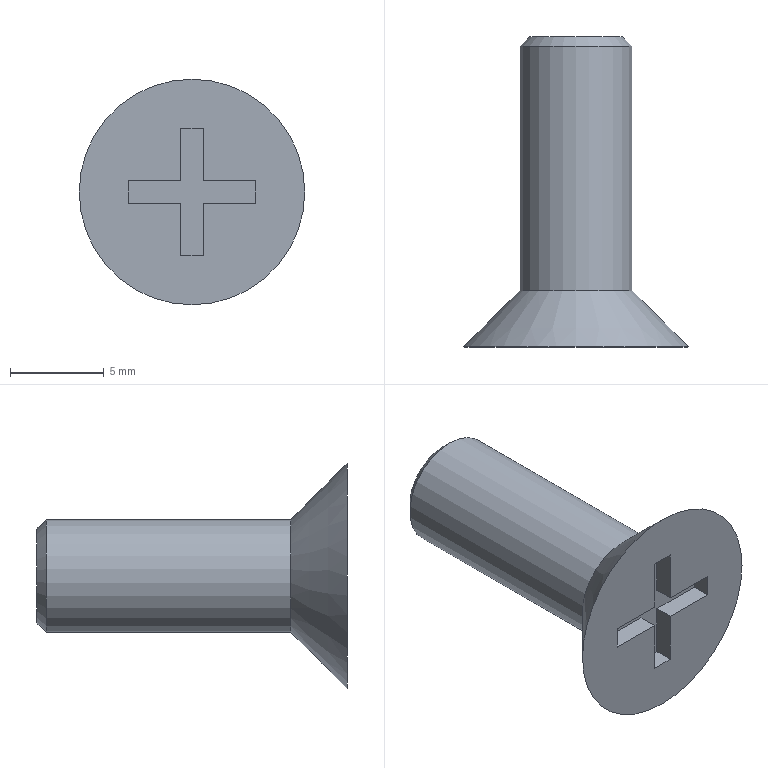Part | NX | features DATUM_CSYS 3, SKETCH 2, CHAMFER 1, EXTRUDE 1, SWP104 1 | 1 solid | 18 faces | box 12 x 16.5 x 12 mm | volume 562.519 mm3 | plane 15 | cone 2 | cylinder 1 | commonest cylinder face diameters 6 x1
STEP:
#1=CARTESIAN_POINT('',(0.,0.,6.));
#2=VERTEX_POINT('',#1);
#3=CARTESIAN_POINT('',(0.,0.,0.));
#4=DIRECTION('',(0.,1.,0.));
#5=DIRECTION('',(0.,0.,1.));
#6=AXIS2_PLACEMENT_3D('',#3,#4,#5);
#7=CIRCLE('',#6,6.);
#8=EDGE_CURVE('',#2,#2,#7,.T.);
#9=ORIENTED_EDGE('',*,*,#8,.F.);
#10=EDGE_LOOP('',(#9));
#11=FACE_BOUND('',#10,.T.);
#12=CARTESIAN_POINT('',(0.6,0.,3.4));
#13=VERTEX_POINT('',#12);
#14=CARTESIAN_POINT('',(-0.6,0.,3.4));
#15=VERTEX_POINT('',#14);
#16=CARTESIAN_POINT('',(0.6,0.,3.4));
#17=DIRECTION('',(-1.,0.,0.));
#18=VECTOR('',#17,1000.);
#19=LINE('',#16,#18);
#20=EDGE_CURVE('',#13,#15,#19,.T.);
#21=ORIENTED_EDGE('',*,*,#20,.F.);
#22=CARTESIAN_POINT('',(0.6,0.,0.6));
#23=VERTEX_POINT('',#22);
#24=CARTESIAN_POINT('',(0.6,0.,0.6));
#25=DIRECTION('',(0.,0.,1.));
#26=VECTOR('',#25,1000.);
#27=LINE('',#24,#26);
#28=EDGE_CURVE('',#23,#13,#27,.T.);
#29=ORIENTED_EDGE('',*,*,#28,.F.);
#30=CARTESIAN_POINT('',(3.4,0.,0.6));
#31=VERTEX_POINT('',#30);
#32=CARTESIAN_POINT('',(3.4,0.,0.6));
#33=DIRECTION('',(-1.,0.,0.));
#34=VECTOR('',#33,1000.);
#35=LINE('',#32,#34);
#36=EDGE_CURVE('',#31,#23,#35,.T.);
#37=ORIENTED_EDGE('',*,*,#36,.F.);
#38=CARTESIAN_POINT('',(3.4,0.,-0.6));
#39=VERTEX_POINT('',#38);
#40=CARTESIAN_POINT('',(3.4,0.,-0.6));
#41=DIRECTION('',(0.,0.,1.));
#42=VECTOR('',#41,1000.);
#43=LINE('',#40,#42);
#44=EDGE_CURVE('',#39,#31,#43,.T.);
#45=ORIENTED_EDGE('',*,*,#44,.F.);
#46=CARTESIAN_POINT('',(0.6,0.,-0.6));
#47=VERTEX_POINT('',#46);
#48=CARTESIAN_POINT('',(0.6,0.,-0.6));
#49=DIRECTION('',(1.,0.,0.));
#50=VECTOR('',#49,1000.);
#51=LINE('',#48,#50);
#52=EDGE_CURVE('',#47,#39,#51,.T.);
#53=ORIENTED_EDGE('',*,*,#52,.F.);
#54=CARTESIAN_POINT('',(0.6,0.,-3.4));
#55=VERTEX_POINT('',#54);
#56=CARTESIAN_POINT('',(0.6,0.,-3.4));
#57=DIRECTION('',(0.,0.,1.));
#58=VECTOR('',#57,1000.);
#59=LINE('',#56,#58);
#60=EDGE_CURVE('',#55,#47,#59,.T.);
#61=ORIENTED_EDGE('',*,*,#60,.F.);
#62=CARTESIAN_POINT('',(-0.6,0.,-3.4));
#63=VERTEX_POINT('',#62);
#64=CARTESIAN_POINT('',(-0.6,0.,-3.4));
#65=DIRECTION('',(1.,0.,0.));
#66=VECTOR('',#65,1000.);
#67=LINE('',#64,#66);
#68=EDGE_CURVE('',#63,#55,#67,.T.);
#69=ORIENTED_EDGE('',*,*,#68,.F.);
#70=CARTESIAN_POINT('',(-0.6,0.,-0.6));
#71=VERTEX_POINT('',#70);
#72=CARTESIAN_POINT('',(-0.6,0.,-0.6));
#73=DIRECTION('',(0.,0.,-1.));
#74=VECTOR('',#73,1000.);
#75=LINE('',#72,#74);
#76=EDGE_CURVE('',#71,#63,#75,.T.);
#77=ORIENTED_EDGE('',*,*,#76,.F.);
#78=CARTESIAN_POINT('',(-3.4,0.,-0.6));
#79=VERTEX_POINT('',#78);
#80=CARTESIAN_POINT('',(-3.4,0.,-0.6));
#81=DIRECTION('',(1.,0.,0.));
#82=VECTOR('',#81,1000.);
#83=LINE('',#80,#82);
#84=EDGE_CURVE('',#79,#71,#83,.T.);
#85=ORIENTED_EDGE('',*,*,#84,.F.);
#86=CARTESIAN_POINT('',(-3.4,0.,0.6));
#87=VERTEX_POINT('',#86);
#88=CARTESIAN_POINT('',(-3.4,0.,0.6));
#89=DIRECTION('',(0.,0.,-1.));
#90=VECTOR('',#89,1000.);
#91=LINE('',#88,#90);
#92=EDGE_CURVE('',#87,#79,#91,.T.);
#93=ORIENTED_EDGE('',*,*,#92,.F.);
#94=CARTESIAN_POINT('',(-0.6,0.,0.6));
#95=VERTEX_POINT('',#94);
#96=CARTESIAN_POINT('',(-0.6,0.,0.6));
#97=DIRECTION('',(-1.,0.,0.));
#98=VECTOR('',#97,1000.);
#99=LINE('',#96,#98);
#100=EDGE_CURVE('',#95,#87,#99,.T.);
#101=ORIENTED_EDGE('',*,*,#100,.F.);
#102=CARTESIAN_POINT('',(-0.6,0.,3.4));
#103=DIRECTION('',(0.,0.,-1.));
#104=VECTOR('',#103,1000.);
#105=LINE('',#102,#104);
#106=EDGE_CURVE('',#15,#95,#105,.T.);
#107=ORIENTED_EDGE('',*,*,#106,.F.);
#108=EDGE_LOOP('',(#21,#29,#37,#45,#53,#61,#69,#77,#85,#93,#101,#107));
#109=FACE_BOUND('',#108,.T.);
#110=CARTESIAN_POINT('',(0.,0.,0.));
#111=DIRECTION('',(0.,1.,0.));
#112=DIRECTION('',(0.,0.,1.));
#113=AXIS2_PLACEMENT_3D('',#110,#111,#112);
#114=PLANE('',#113);
#115=ADVANCED_FACE('',(#11,#109),#114,.F.);
#116=CARTESIAN_POINT('',(0.,3.,3.));
#117=VERTEX_POINT('',#116);
#118=CARTESIAN_POINT('',(0.,3.,0.));
#119=DIRECTION('',(0.,1.,0.));
#120=DIRECTION('',(0.,0.,1.));
#121=AXIS2_PLACEMENT_3D('',#118,#119,#120);
#122=CIRCLE('',#121,3.);
#123=EDGE_CURVE('',#117,#117,#122,.T.);
#124=ORIENTED_EDGE('',*,*,#123,.F.);
#125=EDGE_LOOP('',(#124));
#126=FACE_BOUND('',#125,.T.);
#127=ORIENTED_EDGE('',*,*,#8,.T.);
#128=EDGE_LOOP('',(#127));
#129=FACE_BOUND('',#128,.T.);
#130=CARTESIAN_POINT('',(0.,0.,0.));
#131=DIRECTION('',(0.,-1.,0.));
#132=DIRECTION('',(0.,0.,-1.));
#133=AXIS2_PLACEMENT_3D('',#130,#131,#132);
#134=CONICAL_SURFACE('',#133,6.,0.7854);
#135=ADVANCED_FACE('',(#126,#129),#134,.T.);
#136=CARTESIAN_POINT('',(0.,16.,-3.));
#137=VERTEX_POINT('',#136);
#138=CARTESIAN_POINT('',(0.,16.,0.));
#139=DIRECTION('',(0.,-1.,0.));
#140=DIRECTION('',(0.,0.,-1.));
#141=AXIS2_PLACEMENT_3D('',#138,#139,#140);
#142=CIRCLE('',#141,3.);
#143=EDGE_CURVE('',#137,#137,#142,.T.);
#144=ORIENTED_EDGE('',*,*,#143,.T.);
#145=EDGE_LOOP('',(#144));
#146=FACE_BOUND('',#145,.T.);
#147=ORIENTED_EDGE('',*,*,#123,.T.);
#148=EDGE_LOOP('',(#147));
#149=FACE_BOUND('',#148,.T.);
#150=CARTESIAN_POINT('',(0.,0.,0.));
#151=DIRECTION('',(0.,1.,0.));
#152=DIRECTION('',(0.,0.,1.));
#153=AXIS2_PLACEMENT_3D('',#150,#151,#152);
#154=CYLINDRICAL_SURFACE('',#153,3.);
#155=ADVANCED_FACE('',(#146,#149),#154,.T.);
#156=CARTESIAN_POINT('',(0.,16.5,-2.5));
#157=VERTEX_POINT('',#156);
#158=CARTESIAN_POINT('',(0.,16.5,0.));
#159=DIRECTION('',(0.,-1.,0.));
#160=DIRECTION('',(0.,0.,-1.));
#161=AXIS2_PLACEMENT_3D('',#158,#159,#160);
#162=CIRCLE('',#161,2.5);
#163=EDGE_CURVE('',#157,#157,#162,.F.);
#164=ORIENTED_EDGE('',*,*,#163,.T.);
#165=EDGE_LOOP('',(#164));
#166=FACE_BOUND('',#165,.T.);
#167=CARTESIAN_POINT('',(0.,16.5,3.));
#168=DIRECTION('',(0.,-1.,0.));
#169=DIRECTION('',(0.,0.,-1.));
#170=AXIS2_PLACEMENT_3D('',#167,#168,#169);
#171=PLANE('',#170);
#172=ADVANCED_FACE('',(#166),#171,.F.);
#173=ORIENTED_EDGE('',*,*,#143,.F.);
#174=EDGE_LOOP('',(#173));
#175=FACE_BOUND('',#174,.T.);
#176=ORIENTED_EDGE('',*,*,#163,.F.);
#177=EDGE_LOOP('',(#176));
#178=FACE_BOUND('',#177,.T.);
#179=CARTESIAN_POINT('',(0.,16.5,0.));
#180=DIRECTION('',(0.,-1.,0.));
#181=DIRECTION('',(0.,0.,-1.));
#182=AXIS2_PLACEMENT_3D('',#179,#180,#181);
#183=CONICAL_SURFACE('',#182,2.5,0.7854);
#184=ADVANCED_FACE('',(#175,#178),#183,.T.);
#185=ORIENTED_EDGE('',*,*,#20,.T.);
#186=CARTESIAN_POINT('',(-0.6,1.,3.4));
#187=VERTEX_POINT('',#186);
#188=CARTESIAN_POINT('',(-0.6,1.,3.4));
#189=DIRECTION('',(0.,-1.,0.));
#190=VECTOR('',#189,1000.);
#191=LINE('',#188,#190);
#192=EDGE_CURVE('',#15,#187,#191,.F.);
#193=ORIENTED_EDGE('',*,*,#192,.T.);
#194=CARTESIAN_POINT('',(0.6,1.,3.4));
#195=VERTEX_POINT('',#194);
#196=CARTESIAN_POINT('',(0.6,1.,3.4));
#197=DIRECTION('',(-1.,0.,0.));
#198=VECTOR('',#197,1000.);
#199=LINE('',#196,#198);
#200=EDGE_CURVE('',#187,#195,#199,.F.);
#201=ORIENTED_EDGE('',*,*,#200,.T.);
#202=CARTESIAN_POINT('',(0.6,1.,3.4));
#203=DIRECTION('',(0.,-1.,0.));
#204=VECTOR('',#203,1000.);
#205=LINE('',#202,#204);
#206=EDGE_CURVE('',#13,#195,#205,.F.);
#207=ORIENTED_EDGE('',*,*,#206,.F.);
#208=EDGE_LOOP('',(#185,#193,#201,#207));
#209=FACE_BOUND('',#208,.T.);
#210=CARTESIAN_POINT('',(0.6,1.,3.4));
#211=DIRECTION('',(0.,0.,1.));
#212=DIRECTION('',(1.,0.,0.));
#213=AXIS2_PLACEMENT_3D('',#210,#211,#212);
#214=PLANE('',#213);
#215=ADVANCED_FACE('',(#209),#214,.F.);
#216=ORIENTED_EDGE('',*,*,#106,.T.);
#217=CARTESIAN_POINT('',(-0.6,1.,0.6));
#218=VERTEX_POINT('',#217);
#219=CARTESIAN_POINT('',(-0.6,1.,0.6));
#220=DIRECTION('',(0.,-1.,0.));
#221=VECTOR('',#220,1000.);
#222=LINE('',#219,#221);
#223=EDGE_CURVE('',#95,#218,#222,.F.);
#224=ORIENTED_EDGE('',*,*,#223,.T.);
#225=CARTESIAN_POINT('',(-0.6,1.,3.4));
#226=DIRECTION('',(0.,0.,-1.));
#227=VECTOR('',#226,1000.);
#228=LINE('',#225,#227);
#229=EDGE_CURVE('',#218,#187,#228,.F.);
#230=ORIENTED_EDGE('',*,*,#229,.T.);
#231=ORIENTED_EDGE('',*,*,#192,.F.);
#232=EDGE_LOOP('',(#216,#224,#230,#231));
#233=FACE_BOUND('',#232,.T.);
#234=CARTESIAN_POINT('',(-0.6,1.,3.4));
#235=DIRECTION('',(-1.,0.,0.));
#236=DIRECTION('',(0.,0.,1.));
#237=AXIS2_PLACEMENT_3D('',#234,#235,#236);
#238=PLANE('',#237);
#239=ADVANCED_FACE('',(#233),#238,.F.);
#240=ORIENTED_EDGE('',*,*,#100,.T.);
#241=CARTESIAN_POINT('',(-3.4,1.,0.6));
#242=VERTEX_POINT('',#241);
#243=CARTESIAN_POINT('',(-3.4,1.,0.6));
#244=DIRECTION('',(0.,-1.,0.));
#245=VECTOR('',#244,1000.);
#246=LINE('',#243,#245);
#247=EDGE_CURVE('',#87,#242,#246,.F.);
#248=ORIENTED_EDGE('',*,*,#247,.T.);
#249=CARTESIAN_POINT('',(-0.6,1.,0.6));
#250=DIRECTION('',(-1.,0.,0.));
#251=VECTOR('',#250,1000.);
#252=LINE('',#249,#251);
#253=EDGE_CURVE('',#242,#218,#252,.F.);
#254=ORIENTED_EDGE('',*,*,#253,.T.);
#255=ORIENTED_EDGE('',*,*,#223,.F.);
#256=EDGE_LOOP('',(#240,#248,#254,#255));
#257=FACE_BOUND('',#256,.T.);
#258=CARTESIAN_POINT('',(-0.6,1.,0.6));
#259=DIRECTION('',(0.,0.,1.));
#260=DIRECTION('',(1.,0.,0.));
#261=AXIS2_PLACEMENT_3D('',#258,#259,#260);
#262=PLANE('',#261);
#263=ADVANCED_FACE('',(#257),#262,.F.);
#264=ORIENTED_EDGE('',*,*,#92,.T.);
#265=CARTESIAN_POINT('',(-3.4,1.,-0.6));
#266=VERTEX_POINT('',#265);
#267=CARTESIAN_POINT('',(-3.4,1.,-0.6));
#268=DIRECTION('',(0.,-1.,0.));
#269=VECTOR('',#268,1000.);
#270=LINE('',#267,#269);
#271=EDGE_CURVE('',#79,#266,#270,.F.);
#272=ORIENTED_EDGE('',*,*,#271,.T.);
#273=CARTESIAN_POINT('',(-3.4,1.,0.6));
#274=DIRECTION('',(0.,0.,-1.));
#275=VECTOR('',#274,1000.);
#276=LINE('',#273,#275);
#277=EDGE_CURVE('',#266,#242,#276,.F.);
#278=ORIENTED_EDGE('',*,*,#277,.T.);
#279=ORIENTED_EDGE('',*,*,#247,.F.);
#280=EDGE_LOOP('',(#264,#272,#278,#279));
#281=FACE_BOUND('',#280,.T.);
#282=CARTESIAN_POINT('',(-3.4,1.,0.6));
#283=DIRECTION('',(-1.,0.,0.));
#284=DIRECTION('',(0.,0.,1.));
#285=AXIS2_PLACEMENT_3D('',#282,#283,#284);
#286=PLANE('',#285);
#287=ADVANCED_FACE('',(#281),#286,.F.);
#288=ORIENTED_EDGE('',*,*,#84,.T.);
#289=CARTESIAN_POINT('',(-0.6,1.,-0.6));
#290=VERTEX_POINT('',#289);
#291=CARTESIAN_POINT('',(-0.6,1.,-0.6));
#292=DIRECTION('',(0.,-1.,0.));
#293=VECTOR('',#292,1000.);
#294=LINE('',#291,#293);
#295=EDGE_CURVE('',#71,#290,#294,.F.);
#296=ORIENTED_EDGE('',*,*,#295,.T.);
#297=CARTESIAN_POINT('',(-3.4,1.,-0.6));
#298=DIRECTION('',(1.,0.,0.));
#299=VECTOR('',#298,1000.);
#300=LINE('',#297,#299);
#301=EDGE_CURVE('',#290,#266,#300,.F.);
#302=ORIENTED_EDGE('',*,*,#301,.T.);
#303=ORIENTED_EDGE('',*,*,#271,.F.);
#304=EDGE_LOOP('',(#288,#296,#302,#303));
#305=FACE_BOUND('',#304,.T.);
#306=CARTESIAN_POINT('',(-3.4,1.,-0.6));
#307=DIRECTION('',(0.,0.,-1.));
#308=DIRECTION('',(-1.,0.,0.));
#309=AXIS2_PLACEMENT_3D('',#306,#307,#308);
#310=PLANE('',#309);
#311=ADVANCED_FACE('',(#305),#310,.F.);
#312=ORIENTED_EDGE('',*,*,#76,.T.);
#313=CARTESIAN_POINT('',(-0.6,1.,-3.4));
#314=VERTEX_POINT('',#313);
#315=CARTESIAN_POINT('',(-0.6,1.,-3.4));
#316=DIRECTION('',(0.,-1.,0.));
#317=VECTOR('',#316,1000.);
#318=LINE('',#315,#317);
#319=EDGE_CURVE('',#63,#314,#318,.F.);
#320=ORIENTED_EDGE('',*,*,#319,.T.);
#321=CARTESIAN_POINT('',(-0.6,1.,-0.6));
#322=DIRECTION('',(0.,0.,-1.));
#323=VECTOR('',#322,1000.);
#324=LINE('',#321,#323);
#325=EDGE_CURVE('',#314,#290,#324,.F.);
#326=ORIENTED_EDGE('',*,*,#325,.T.);
#327=ORIENTED_EDGE('',*,*,#295,.F.);
#328=EDGE_LOOP('',(#312,#320,#326,#327));
#329=FACE_BOUND('',#328,.T.);
#330=CARTESIAN_POINT('',(-0.6,1.,-0.6));
#331=DIRECTION('',(-1.,0.,0.));
#332=DIRECTION('',(0.,0.,1.));
#333=AXIS2_PLACEMENT_3D('',#330,#331,#332);
#334=PLANE('',#333);
#335=ADVANCED_FACE('',(#329),#334,.F.);
#336=ORIENTED_EDGE('',*,*,#68,.T.);
#337=CARTESIAN_POINT('',(0.6,1.,-3.4));
#338=VERTEX_POINT('',#337);
#339=CARTESIAN_POINT('',(0.6,1.,-3.4));
#340=DIRECTION('',(0.,-1.,0.));
#341=VECTOR('',#340,1000.);
#342=LINE('',#339,#341);
#343=EDGE_CURVE('',#55,#338,#342,.F.);
#344=ORIENTED_EDGE('',*,*,#343,.T.);
#345=CARTESIAN_POINT('',(-0.6,1.,-3.4));
#346=DIRECTION('',(1.,0.,0.));
#347=VECTOR('',#346,1000.);
#348=LINE('',#345,#347);
#349=EDGE_CURVE('',#338,#314,#348,.F.);
#350=ORIENTED_EDGE('',*,*,#349,.T.);
#351=ORIENTED_EDGE('',*,*,#319,.F.);
#352=EDGE_LOOP('',(#336,#344,#350,#351));
#353=FACE_BOUND('',#352,.T.);
#354=CARTESIAN_POINT('',(-0.6,1.,-3.4));
#355=DIRECTION('',(0.,0.,-1.));
#356=DIRECTION('',(-1.,0.,0.));
#357=AXIS2_PLACEMENT_3D('',#354,#355,#356);
#358=PLANE('',#357);
#359=ADVANCED_FACE('',(#353),#358,.F.);
#360=ORIENTED_EDGE('',*,*,#60,.T.);
#361=CARTESIAN_POINT('',(0.6,1.,-0.6));
#362=VERTEX_POINT('',#361);
#363=CARTESIAN_POINT('',(0.6,1.,-0.6));
#364=DIRECTION('',(0.,-1.,0.));
#365=VECTOR('',#364,1000.);
#366=LINE('',#363,#365);
#367=EDGE_CURVE('',#47,#362,#366,.F.);
#368=ORIENTED_EDGE('',*,*,#367,.T.);
#369=CARTESIAN_POINT('',(0.6,1.,-3.4));
#370=DIRECTION('',(0.,0.,1.));
#371=VECTOR('',#370,1000.);
#372=LINE('',#369,#371);
#373=EDGE_CURVE('',#362,#338,#372,.F.);
#374=ORIENTED_EDGE('',*,*,#373,.T.);
#375=ORIENTED_EDGE('',*,*,#343,.F.);
#376=EDGE_LOOP('',(#360,#368,#374,#375));
#377=FACE_BOUND('',#376,.T.);
#378=CARTESIAN_POINT('',(0.6,1.,-3.4));
#379=DIRECTION('',(1.,0.,0.));
#380=DIRECTION('',(0.,0.,-1.));
#381=AXIS2_PLACEMENT_3D('',#378,#379,#380);
#382=PLANE('',#381);
#383=ADVANCED_FACE('',(#377),#382,.F.);
#384=ORIENTED_EDGE('',*,*,#52,.T.);
#385=CARTESIAN_POINT('',(3.4,1.,-0.6));
#386=VERTEX_POINT('',#385);
#387=CARTESIAN_POINT('',(3.4,1.,-0.6));
#388=DIRECTION('',(0.,-1.,0.));
#389=VECTOR('',#388,1000.);
#390=LINE('',#387,#389);
#391=EDGE_CURVE('',#39,#386,#390,.F.);
#392=ORIENTED_EDGE('',*,*,#391,.T.);
#393=CARTESIAN_POINT('',(0.6,1.,-0.6));
#394=DIRECTION('',(1.,0.,0.));
#395=VECTOR('',#394,1000.);
#396=LINE('',#393,#395);
#397=EDGE_CURVE('',#386,#362,#396,.F.);
#398=ORIENTED_EDGE('',*,*,#397,.T.);
#399=ORIENTED_EDGE('',*,*,#367,.F.);
#400=EDGE_LOOP('',(#384,#392,#398,#399));
#401=FACE_BOUND('',#400,.T.);
#402=CARTESIAN_POINT('',(0.6,1.,-0.6));
#403=DIRECTION('',(0.,0.,-1.));
#404=DIRECTION('',(-1.,0.,0.));
#405=AXIS2_PLACEMENT_3D('',#402,#403,#404);
#406=PLANE('',#405);
#407=ADVANCED_FACE('',(#401),#406,.F.);
#408=ORIENTED_EDGE('',*,*,#44,.T.);
#409=CARTESIAN_POINT('',(3.4,1.,0.6));
#410=VERTEX_POINT('',#409);
#411=CARTESIAN_POINT('',(3.4,1.,0.6));
#412=DIRECTION('',(0.,-1.,0.));
#413=VECTOR('',#412,1000.);
#414=LINE('',#411,#413);
#415=EDGE_CURVE('',#31,#410,#414,.F.);
#416=ORIENTED_EDGE('',*,*,#415,.T.);
#417=CARTESIAN_POINT('',(3.4,1.,-0.6));
#418=DIRECTION('',(0.,0.,1.));
#419=VECTOR('',#418,1000.);
#420=LINE('',#417,#419);
#421=EDGE_CURVE('',#410,#386,#420,.F.);
#422=ORIENTED_EDGE('',*,*,#421,.T.);
#423=ORIENTED_EDGE('',*,*,#391,.F.);
#424=EDGE_LOOP('',(#408,#416,#422,#423));
#425=FACE_BOUND('',#424,.T.);
#426=CARTESIAN_POINT('',(3.4,1.,-0.6));
#427=DIRECTION('',(1.,0.,0.));
#428=DIRECTION('',(0.,0.,-1.));
#429=AXIS2_PLACEMENT_3D('',#426,#427,#428);
#430=PLANE('',#429);
#431=ADVANCED_FACE('',(#425),#430,.F.);
#432=ORIENTED_EDGE('',*,*,#36,.T.);
#433=CARTESIAN_POINT('',(0.6,1.,0.6));
#434=VERTEX_POINT('',#433);
#435=CARTESIAN_POINT('',(0.6,1.,0.6));
#436=DIRECTION('',(0.,-1.,0.));
#437=VECTOR('',#436,1000.);
#438=LINE('',#435,#437);
#439=EDGE_CURVE('',#23,#434,#438,.F.);
#440=ORIENTED_EDGE('',*,*,#439,.T.);
#441=CARTESIAN_POINT('',(3.4,1.,0.6));
#442=DIRECTION('',(-1.,0.,0.));
#443=VECTOR('',#442,1000.);
#444=LINE('',#441,#443);
#445=EDGE_CURVE('',#434,#410,#444,.F.);
#446=ORIENTED_EDGE('',*,*,#445,.T.);
#447=ORIENTED_EDGE('',*,*,#415,.F.);
#448=EDGE_LOOP('',(#432,#440,#446,#447));
#449=FACE_BOUND('',#448,.T.);
#450=CARTESIAN_POINT('',(3.4,1.,0.6));
#451=DIRECTION('',(0.,0.,1.));
#452=DIRECTION('',(1.,0.,0.));
#453=AXIS2_PLACEMENT_3D('',#450,#451,#452);
#454=PLANE('',#453);
#455=ADVANCED_FACE('',(#449),#454,.F.);
#456=ORIENTED_EDGE('',*,*,#28,.T.);
#457=ORIENTED_EDGE('',*,*,#206,.T.);
#458=CARTESIAN_POINT('',(0.6,1.,0.6));
#459=DIRECTION('',(0.,0.,1.));
#460=VECTOR('',#459,1000.);
#461=LINE('',#458,#460);
#462=EDGE_CURVE('',#195,#434,#461,.F.);
#463=ORIENTED_EDGE('',*,*,#462,.T.);
#464=ORIENTED_EDGE('',*,*,#439,.F.);
#465=EDGE_LOOP('',(#456,#457,#463,#464));
#466=FACE_BOUND('',#465,.T.);
#467=CARTESIAN_POINT('',(0.6,1.,0.6));
#468=DIRECTION('',(1.,0.,0.));
#469=DIRECTION('',(0.,0.,-1.));
#470=AXIS2_PLACEMENT_3D('',#467,#468,#469);
#471=PLANE('',#470);
#472=ADVANCED_FACE('',(#466),#471,.F.);
#473=ORIENTED_EDGE('',*,*,#200,.F.);
#474=ORIENTED_EDGE('',*,*,#229,.F.);
#475=ORIENTED_EDGE('',*,*,#253,.F.);
#476=ORIENTED_EDGE('',*,*,#277,.F.);
#477=ORIENTED_EDGE('',*,*,#301,.F.);
#478=ORIENTED_EDGE('',*,*,#325,.F.);
#479=ORIENTED_EDGE('',*,*,#349,.F.);
#480=ORIENTED_EDGE('',*,*,#373,.F.);
#481=ORIENTED_EDGE('',*,*,#397,.F.);
#482=ORIENTED_EDGE('',*,*,#421,.F.);
#483=ORIENTED_EDGE('',*,*,#445,.F.);
#484=ORIENTED_EDGE('',*,*,#462,.F.);
#485=EDGE_LOOP('',(#473,#474,#475,#476,#477,#478,#479,#480,#481,#482,#483,#484));
#486=FACE_BOUND('',#485,.T.);
#487=CARTESIAN_POINT('',(0.,1.,0.));
#488=DIRECTION('',(0.,-1.,0.));
#489=DIRECTION('',(0.,0.,-1.));
#490=AXIS2_PLACEMENT_3D('',#487,#488,#489);
#491=PLANE('',#490);
#492=ADVANCED_FACE('',(#486),#491,.T.);
#493=CLOSED_SHELL('',(#115,#135,#155,#172,#184,#215,#239,#263,#287,#311,#335,#359,#383,#407,#431,#455,#472,#492));
#494=MANIFOLD_SOLID_BREP('',#493);
#495=(LENGTH_UNIT()NAMED_UNIT(*)SI_UNIT(.MILLI.,.METRE.));
#496=UNCERTAINTY_MEASURE_WITH_UNIT(LENGTH_MEASURE(0.00001),#495,'','');
#497=(NAMED_UNIT(*)PLANE_ANGLE_UNIT()SI_UNIT($,.RADIAN.));
#498=(NAMED_UNIT(*)SI_UNIT($,.STERADIAN.)SOLID_ANGLE_UNIT());
#499=(GEOMETRIC_REPRESENTATION_CONTEXT(3)GLOBAL_UNCERTAINTY_ASSIGNED_CONTEXT((#496))GLOBAL_UNIT_ASSIGNED_CONTEXT((#495,#497,#498))REPRESENTATION_CONTEXT('',''));
#500=ADVANCED_BREP_SHAPE_REPRESENTATION('',(#494),#499);